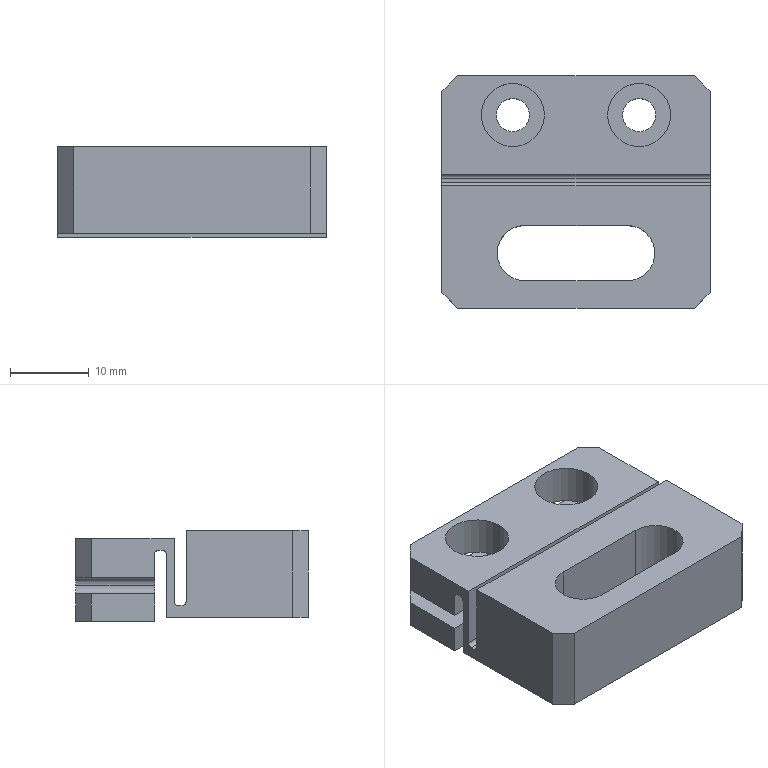Part | SolidWorks | features MoveFace 11, Cut 3, DelFace 2, Fillet 2, BaseBody 1, ICE 1 | 1 solid | 47 faces | box 34 x 29.5 x 11.5 mm | volume 7154 mm3 | plane 28 | cylinder 19 | commonest cylinder face diameters 1 x4 2 x4 4.2 x4 8 x4 7 x3
STEP:
#1=CARTESIAN_POINT('',(4.,8.75,9.));
#2=VERTEX_POINT('',#1);
#3=CARTESIAN_POINT('',(12.,8.75,9.));
#4=VERTEX_POINT('',#3);
#5=CARTESIAN_POINT('',(8.,8.75,9.));
#6=DIRECTION('',(0.,0.,1.));
#7=DIRECTION('',(1.,0.,0.));
#8=AXIS2_PLACEMENT_3D('',#5,#6,#7);
#9=CIRCLE('',#8,4.);
#10=EDGE_CURVE('',#2,#4,#9,.T.);
#11=ORIENTED_EDGE('',*,*,#10,.F.);
#12=CARTESIAN_POINT('',(4.,8.75,14.));
#13=VERTEX_POINT('',#12);
#14=CARTESIAN_POINT('',(4.,8.75,8.));
#15=DIRECTION('',(0.,0.,1.));
#16=VECTOR('',#15,1000.);
#17=LINE('',#14,#16);
#18=EDGE_CURVE('',#2,#13,#17,.T.);
#19=ORIENTED_EDGE('',*,*,#18,.T.);
#20=CARTESIAN_POINT('',(12.,8.75,14.));
#21=VERTEX_POINT('',#20);
#22=CARTESIAN_POINT('',(8.,8.75,14.));
#23=DIRECTION('',(0.,0.,1.));
#24=DIRECTION('',(1.,0.,0.));
#25=AXIS2_PLACEMENT_3D('',#22,#23,#24);
#26=CIRCLE('',#25,4.);
#27=EDGE_CURVE('',#13,#21,#26,.T.);
#28=ORIENTED_EDGE('',*,*,#27,.T.);
#29=CARTESIAN_POINT('',(12.,8.75,8.));
#30=DIRECTION('',(0.,0.,1.));
#31=VECTOR('',#30,1000.);
#32=LINE('',#29,#31);
#33=EDGE_CURVE('',#4,#21,#32,.T.);
#34=ORIENTED_EDGE('',*,*,#33,.F.);
#35=EDGE_LOOP('',(#11,#19,#28,#34));
#36=FACE_OUTER_BOUND('',#35,.T.);
#37=CARTESIAN_POINT('',(8.,8.75,8.));
#38=DIRECTION('',(0.,0.,1.));
#39=DIRECTION('',(1.,0.,0.));
#40=AXIS2_PLACEMENT_3D('',#37,#38,#39);
#41=CYLINDRICAL_SURFACE('',#40,4.);
#42=ADVANCED_FACE('',(#36),#41,.F.);
#43=CARTESIAN_POINT('',(-12.,8.75,9.));
#44=VERTEX_POINT('',#43);
#45=CARTESIAN_POINT('',(-4.,8.75,9.));
#46=VERTEX_POINT('',#45);
#47=CARTESIAN_POINT('',(-8.,8.75,9.));
#48=DIRECTION('',(0.,0.,1.));
#49=DIRECTION('',(1.,0.,0.));
#50=AXIS2_PLACEMENT_3D('',#47,#48,#49);
#51=CIRCLE('',#50,4.);
#52=EDGE_CURVE('',#44,#46,#51,.T.);
#53=ORIENTED_EDGE('',*,*,#52,.F.);
#54=CARTESIAN_POINT('',(-12.,8.75,14.));
#55=VERTEX_POINT('',#54);
#56=CARTESIAN_POINT('',(-12.,8.75,8.));
#57=DIRECTION('',(0.,0.,1.));
#58=VECTOR('',#57,1000.);
#59=LINE('',#56,#58);
#60=EDGE_CURVE('',#44,#55,#59,.T.);
#61=ORIENTED_EDGE('',*,*,#60,.T.);
#62=CARTESIAN_POINT('',(-4.,8.75,14.));
#63=VERTEX_POINT('',#62);
#64=CARTESIAN_POINT('',(-8.,8.75,14.));
#65=DIRECTION('',(0.,0.,1.));
#66=DIRECTION('',(1.,0.,0.));
#67=AXIS2_PLACEMENT_3D('',#64,#65,#66);
#68=CIRCLE('',#67,4.);
#69=EDGE_CURVE('',#55,#63,#68,.T.);
#70=ORIENTED_EDGE('',*,*,#69,.T.);
#71=CARTESIAN_POINT('',(-4.,8.75,8.));
#72=DIRECTION('',(0.,0.,1.));
#73=VECTOR('',#72,1000.);
#74=LINE('',#71,#73);
#75=EDGE_CURVE('',#46,#63,#74,.T.);
#76=ORIENTED_EDGE('',*,*,#75,.F.);
#77=EDGE_LOOP('',(#53,#61,#70,#76));
#78=FACE_OUTER_BOUND('',#77,.T.);
#79=CARTESIAN_POINT('',(-8.,8.75,8.));
#80=DIRECTION('',(0.,0.,1.));
#81=DIRECTION('',(1.,0.,0.));
#82=AXIS2_PLACEMENT_3D('',#79,#80,#81);
#83=CYLINDRICAL_SURFACE('',#82,4.);
#84=ADVANCED_FACE('',(#78),#83,.F.);
#85=CARTESIAN_POINT('',(-5.9,8.75,3.5));
#86=VERTEX_POINT('',#85);
#87=CARTESIAN_POINT('',(-10.1,8.75,3.5));
#88=VERTEX_POINT('',#87);
#89=CARTESIAN_POINT('',(-8.,8.75,3.5));
#90=DIRECTION('',(0.,0.,-1.));
#91=DIRECTION('',(-1.,0.,0.));
#92=AXIS2_PLACEMENT_3D('',#89,#90,#91);
#93=CIRCLE('',#92,2.1);
#94=EDGE_CURVE('',#86,#88,#93,.T.);
#95=ORIENTED_EDGE('',*,*,#94,.T.);
#96=CARTESIAN_POINT('',(-10.1,8.75,7.));
#97=VERTEX_POINT('',#96);
#98=CARTESIAN_POINT('',(-10.1,8.75,-6.));
#99=DIRECTION('',(0.,0.,1.));
#100=VECTOR('',#99,1000.);
#101=LINE('',#98,#100);
#102=EDGE_CURVE('',#88,#97,#101,.T.);
#103=ORIENTED_EDGE('',*,*,#102,.T.);
#104=CARTESIAN_POINT('',(-5.9,8.75,7.));
#105=VERTEX_POINT('',#104);
#106=CARTESIAN_POINT('',(-8.,8.75,7.));
#107=DIRECTION('',(0.,0.,-1.));
#108=DIRECTION('',(-1.,0.,0.));
#109=AXIS2_PLACEMENT_3D('',#106,#107,#108);
#110=CIRCLE('',#109,2.1);
#111=EDGE_CURVE('',#105,#97,#110,.T.);
#112=ORIENTED_EDGE('',*,*,#111,.F.);
#113=CARTESIAN_POINT('',(-5.9,8.75,-6.));
#114=DIRECTION('',(0.,0.,1.));
#115=VECTOR('',#114,1000.);
#116=LINE('',#113,#115);
#117=EDGE_CURVE('',#86,#105,#116,.T.);
#118=ORIENTED_EDGE('',*,*,#117,.F.);
#119=EDGE_LOOP('',(#95,#103,#112,#118));
#120=FACE_OUTER_BOUND('',#119,.T.);
#121=CARTESIAN_POINT('',(-8.,8.75,-6.));
#122=DIRECTION('',(0.,0.,1.));
#123=DIRECTION('',(1.,0.,0.));
#124=AXIS2_PLACEMENT_3D('',#121,#122,#123);
#125=CYLINDRICAL_SURFACE('',#124,2.1);
#126=ADVANCED_FACE('',(#120),#125,.F.);
#127=CARTESIAN_POINT('',(10.1,8.75,3.5));
#128=VERTEX_POINT('',#127);
#129=CARTESIAN_POINT('',(5.9,8.75,3.5));
#130=VERTEX_POINT('',#129);
#131=CARTESIAN_POINT('',(8.,8.75,3.5));
#132=DIRECTION('',(0.,0.,-1.));
#133=DIRECTION('',(-1.,0.,0.));
#134=AXIS2_PLACEMENT_3D('',#131,#132,#133);
#135=CIRCLE('',#134,2.1);
#136=EDGE_CURVE('',#128,#130,#135,.T.);
#137=ORIENTED_EDGE('',*,*,#136,.T.);
#138=CARTESIAN_POINT('',(5.9,8.75,7.));
#139=VERTEX_POINT('',#138);
#140=CARTESIAN_POINT('',(5.9,8.75,-6.));
#141=DIRECTION('',(0.,0.,1.));
#142=VECTOR('',#141,1000.);
#143=LINE('',#140,#142);
#144=EDGE_CURVE('',#130,#139,#143,.T.);
#145=ORIENTED_EDGE('',*,*,#144,.T.);
#146=CARTESIAN_POINT('',(10.1,8.75,7.));
#147=VERTEX_POINT('',#146);
#148=CARTESIAN_POINT('',(8.,8.75,7.));
#149=DIRECTION('',(0.,0.,-1.));
#150=DIRECTION('',(-1.,0.,0.));
#151=AXIS2_PLACEMENT_3D('',#148,#149,#150);
#152=CIRCLE('',#151,2.1);
#153=EDGE_CURVE('',#147,#139,#152,.T.);
#154=ORIENTED_EDGE('',*,*,#153,.F.);
#155=CARTESIAN_POINT('',(10.1,8.75,-6.));
#156=DIRECTION('',(0.,0.,1.));
#157=VECTOR('',#156,1000.);
#158=LINE('',#155,#157);
#159=EDGE_CURVE('',#128,#147,#158,.T.);
#160=ORIENTED_EDGE('',*,*,#159,.F.);
#161=EDGE_LOOP('',(#137,#145,#154,#160));
#162=FACE_OUTER_BOUND('',#161,.T.);
#163=CARTESIAN_POINT('',(8.,8.75,-6.));
#164=DIRECTION('',(0.,0.,1.));
#165=DIRECTION('',(1.,0.,0.));
#166=AXIS2_PLACEMENT_3D('',#163,#164,#165);
#167=CYLINDRICAL_SURFACE('',#166,2.1);
#168=ADVANCED_FACE('',(#162),#167,.F.);
#169=CARTESIAN_POINT('',(-6.5,-5.25,15.));
#170=VERTEX_POINT('',#169);
#171=CARTESIAN_POINT('',(-10.,-8.75,15.));
#172=VERTEX_POINT('',#171);
#173=CARTESIAN_POINT('',(-6.5,-8.75,15.));
#174=DIRECTION('',(0.,0.,1.));
#175=DIRECTION('',(-1.,0.,0.));
#176=AXIS2_PLACEMENT_3D('',#173,#174,#175);
#177=CIRCLE('',#176,3.5);
#178=EDGE_CURVE('',#170,#172,#177,.T.);
#179=ORIENTED_EDGE('',*,*,#178,.T.);
#180=CARTESIAN_POINT('',(-10.,-8.75,4.));
#181=VERTEX_POINT('',#180);
#182=CARTESIAN_POINT('',(-10.,-8.75,18.));
#183=DIRECTION('',(0.,0.,-1.));
#184=VECTOR('',#183,1000.);
#185=LINE('',#182,#184);
#186=EDGE_CURVE('',#172,#181,#185,.T.);
#187=ORIENTED_EDGE('',*,*,#186,.T.);
#188=CARTESIAN_POINT('',(-6.5,-5.25,4.));
#189=VERTEX_POINT('',#188);
#190=CARTESIAN_POINT('',(-6.5,-8.75,4.));
#191=DIRECTION('',(0.,0.,-1.));
#192=DIRECTION('',(1.,0.,0.));
#193=AXIS2_PLACEMENT_3D('',#190,#191,#192);
#194=CIRCLE('',#193,3.5);
#195=EDGE_CURVE('',#181,#189,#194,.T.);
#196=ORIENTED_EDGE('',*,*,#195,.T.);
#197=CARTESIAN_POINT('',(-6.5,-5.25,18.));
#198=DIRECTION('',(0.,0.,-1.));
#199=VECTOR('',#198,1000.);
#200=LINE('',#197,#199);
#201=EDGE_CURVE('',#170,#189,#200,.T.);
#202=ORIENTED_EDGE('',*,*,#201,.F.);
#203=EDGE_LOOP('',(#179,#187,#196,#202));
#204=FACE_OUTER_BOUND('',#203,.T.);
#205=CARTESIAN_POINT('',(-6.5,-8.75,18.));
#206=DIRECTION('',(0.,0.,-1.));
#207=DIRECTION('',(-1.,0.,0.));
#208=AXIS2_PLACEMENT_3D('',#205,#206,#207);
#209=CYLINDRICAL_SURFACE('',#208,3.5);
#210=ADVANCED_FACE('',(#204),#209,.F.);
#211=CARTESIAN_POINT('',(8.,8.75,14.));
#212=DIRECTION('',(0.,0.,1.));
#213=DIRECTION('',(1.,0.,0.));
#214=AXIS2_PLACEMENT_3D('',#211,#212,#213);
#215=CIRCLE('',#214,4.);
#216=EDGE_CURVE('',#21,#13,#215,.T.);
#217=ORIENTED_EDGE('',*,*,#216,.F.);
#218=ORIENTED_EDGE('',*,*,#27,.F.);
#219=EDGE_LOOP('',(#217,#218));
#220=FACE_BOUND('',#219,.T.);
#221=CARTESIAN_POINT('',(-8.,8.75,14.));
#222=DIRECTION('',(0.,0.,1.));
#223=DIRECTION('',(1.,0.,0.));
#224=AXIS2_PLACEMENT_3D('',#221,#222,#223);
#225=CIRCLE('',#224,4.);
#226=EDGE_CURVE('',#63,#55,#225,.T.);
#227=ORIENTED_EDGE('',*,*,#226,.F.);
#228=ORIENTED_EDGE('',*,*,#69,.F.);
#229=EDGE_LOOP('',(#227,#228));
#230=FACE_BOUND('',#229,.T.);
#231=CARTESIAN_POINT('',(15.,13.75,14.));
#232=VERTEX_POINT('',#231);
#233=CARTESIAN_POINT('',(17.,11.75,14.));
#234=VERTEX_POINT('',#233);
#235=CARTESIAN_POINT('',(15.,13.75,14.));
#236=DIRECTION('',(0.7071,-0.7071,0.));
#237=VECTOR('',#236,1000.);
#238=LINE('',#235,#237);
#239=EDGE_CURVE('',#232,#234,#238,.T.);
#240=ORIENTED_EDGE('',*,*,#239,.F.);
#241=CARTESIAN_POINT('',(-15.,13.75,14.));
#242=VERTEX_POINT('',#241);
#243=CARTESIAN_POINT('',(-50.,13.75,14.));
#244=DIRECTION('',(1.,0.,0.));
#245=VECTOR('',#244,1000.);
#246=LINE('',#243,#245);
#247=EDGE_CURVE('',#242,#232,#246,.T.);
#248=ORIENTED_EDGE('',*,*,#247,.F.);
#249=CARTESIAN_POINT('',(-17.,11.75,14.));
#250=VERTEX_POINT('',#249);
#251=CARTESIAN_POINT('',(-17.,11.75,14.));
#252=DIRECTION('',(0.7071,0.7071,0.));
#253=VECTOR('',#252,1000.);
#254=LINE('',#251,#253);
#255=EDGE_CURVE('',#250,#242,#254,.T.);
#256=ORIENTED_EDGE('',*,*,#255,.F.);
#257=CARTESIAN_POINT('',(-17.,1.25,14.));
#258=VERTEX_POINT('',#257);
#259=CARTESIAN_POINT('',(-17.,18.75,14.));
#260=DIRECTION('',(0.,1.,0.));
#261=VECTOR('',#260,1000.);
#262=LINE('',#259,#261);
#263=EDGE_CURVE('',#258,#250,#262,.T.);
#264=ORIENTED_EDGE('',*,*,#263,.F.);
#265=CARTESIAN_POINT('',(17.,1.25,14.));
#266=VERTEX_POINT('',#265);
#267=CARTESIAN_POINT('',(-50.,1.25,14.));
#268=DIRECTION('',(-1.,0.,0.));
#269=VECTOR('',#268,1000.);
#270=LINE('',#267,#269);
#271=EDGE_CURVE('',#266,#258,#270,.T.);
#272=ORIENTED_EDGE('',*,*,#271,.F.);
#273=CARTESIAN_POINT('',(17.,18.75,14.));
#274=DIRECTION('',(0.,-1.,0.));
#275=VECTOR('',#274,1000.);
#276=LINE('',#273,#275);
#277=EDGE_CURVE('',#234,#266,#276,.T.);
#278=ORIENTED_EDGE('',*,*,#277,.F.);
#279=EDGE_LOOP('',(#240,#248,#256,#264,#272,#278));
#280=FACE_OUTER_BOUND('',#279,.T.);
#281=CARTESIAN_POINT('',(-50.,18.75,14.));
#282=DIRECTION('',(0.,0.,-1.));
#283=DIRECTION('',(0.,1.,0.));
#284=AXIS2_PLACEMENT_3D('',#281,#282,#283);
#285=PLANE('',#284);
#286=ADVANCED_FACE('',(#220,#230,#280),#285,.F.);
#287=CARTESIAN_POINT('',(17.,-13.75,4.));
#288=VERTEX_POINT('',#287);
#289=CARTESIAN_POINT('',(17.,-13.75,15.));
#290=VERTEX_POINT('',#289);
#291=CARTESIAN_POINT('',(17.,-13.75,18.));
#292=DIRECTION('',(0.,0.,1.));
#293=VECTOR('',#292,1000.);
#294=LINE('',#291,#293);
#295=EDGE_CURVE('',#288,#290,#294,.T.);
#296=ORIENTED_EDGE('',*,*,#295,.F.);
#297=CARTESIAN_POINT('',(17.,2.25,4.));
#298=VERTEX_POINT('',#297);
#299=CARTESIAN_POINT('',(17.,2.25,4.));
#300=DIRECTION('',(0.,-1.,0.));
#301=VECTOR('',#300,1000.);
#302=LINE('',#299,#301);
#303=EDGE_CURVE('',#298,#288,#302,.T.);
#304=ORIENTED_EDGE('',*,*,#303,.F.);
#305=CARTESIAN_POINT('',(17.,2.25,12.));
#306=VERTEX_POINT('',#305);
#307=CARTESIAN_POINT('',(17.,2.25,18.));
#308=DIRECTION('',(0.,0.,-1.));
#309=VECTOR('',#308,1000.);
#310=LINE('',#307,#309);
#311=EDGE_CURVE('',#306,#298,#310,.T.);
#312=ORIENTED_EDGE('',*,*,#311,.F.);
#313=CARTESIAN_POINT('',(17.,2.75,12.5));
#314=VERTEX_POINT('',#313);
#315=CARTESIAN_POINT('',(17.,2.75,12.));
#316=DIRECTION('',(-1.,0.,0.));
#317=DIRECTION('',(0.,0.,1.));
#318=AXIS2_PLACEMENT_3D('',#315,#316,#317);
#319=CIRCLE('',#318,0.5);
#320=EDGE_CURVE('',#306,#314,#319,.T.);
#321=ORIENTED_EDGE('',*,*,#320,.T.);
#322=CARTESIAN_POINT('',(17.,3.25,12.5));
#323=VERTEX_POINT('',#322);
#324=CARTESIAN_POINT('',(17.,3.75,12.5));
#325=DIRECTION('',(0.,1.,0.));
#326=VECTOR('',#325,1000.);
#327=LINE('',#324,#326);
#328=EDGE_CURVE('',#314,#323,#327,.T.);
#329=ORIENTED_EDGE('',*,*,#328,.T.);
#330=CARTESIAN_POINT('',(17.,3.75,12.));
#331=VERTEX_POINT('',#330);
#332=CARTESIAN_POINT('',(17.,3.25,12.));
#333=DIRECTION('',(-1.,0.,0.));
#334=DIRECTION('',(0.,0.,1.));
#335=AXIS2_PLACEMENT_3D('',#332,#333,#334);
#336=CIRCLE('',#335,0.5);
#337=EDGE_CURVE('',#323,#331,#336,.T.);
#338=ORIENTED_EDGE('',*,*,#337,.T.);
#339=CARTESIAN_POINT('',(17.,3.75,9.));
#340=VERTEX_POINT('',#339);
#341=CARTESIAN_POINT('',(17.,3.75,18.));
#342=DIRECTION('',(0.,0.,1.));
#343=VECTOR('',#342,1000.);
#344=LINE('',#341,#343);
#345=EDGE_CURVE('',#340,#331,#344,.T.);
#346=ORIENTED_EDGE('',*,*,#345,.F.);
#347=CARTESIAN_POINT('',(17.,11.75,9.));
#348=VERTEX_POINT('',#347);
#349=CARTESIAN_POINT('',(17.,-18.75,9.));
#350=DIRECTION('',(0.,-1.,0.));
#351=VECTOR('',#350,1000.);
#352=LINE('',#349,#351);
#353=EDGE_CURVE('',#348,#340,#352,.T.);
#354=ORIENTED_EDGE('',*,*,#353,.F.);
#355=CARTESIAN_POINT('',(17.,11.75,18.));
#356=DIRECTION('',(0.,0.,-1.));
#357=VECTOR('',#356,1000.);
#358=LINE('',#355,#357);
#359=EDGE_CURVE('',#234,#348,#358,.T.);
#360=ORIENTED_EDGE('',*,*,#359,.F.);
#361=ORIENTED_EDGE('',*,*,#277,.T.);
#362=CARTESIAN_POINT('',(17.,1.25,6.));
#363=VERTEX_POINT('',#362);
#364=CARTESIAN_POINT('',(17.,1.25,18.));
#365=DIRECTION('',(0.,0.,1.));
#366=VECTOR('',#365,1000.);
#367=LINE('',#364,#366);
#368=EDGE_CURVE('',#363,#266,#367,.T.);
#369=ORIENTED_EDGE('',*,*,#368,.F.);
#370=CARTESIAN_POINT('',(17.,0.75,5.5));
#371=VERTEX_POINT('',#370);
#372=CARTESIAN_POINT('',(17.,0.75,6.));
#373=DIRECTION('',(-1.,0.,0.));
#374=DIRECTION('',(0.,0.,1.));
#375=AXIS2_PLACEMENT_3D('',#372,#373,#374);
#376=CIRCLE('',#375,0.5);
#377=EDGE_CURVE('',#363,#371,#376,.T.);
#378=ORIENTED_EDGE('',*,*,#377,.T.);
#379=CARTESIAN_POINT('',(17.,0.25,5.5));
#380=VERTEX_POINT('',#379);
#381=CARTESIAN_POINT('',(17.,0.75,5.5));
#382=DIRECTION('',(0.,-1.,0.));
#383=VECTOR('',#382,1000.);
#384=LINE('',#381,#383);
#385=EDGE_CURVE('',#371,#380,#384,.T.);
#386=ORIENTED_EDGE('',*,*,#385,.T.);
#387=CARTESIAN_POINT('',(17.,-0.25,6.));
#388=VERTEX_POINT('',#387);
#389=CARTESIAN_POINT('',(17.,0.25,6.));
#390=DIRECTION('',(-1.,0.,0.));
#391=DIRECTION('',(0.,0.,1.));
#392=AXIS2_PLACEMENT_3D('',#389,#390,#391);
#393=CIRCLE('',#392,0.5);
#394=EDGE_CURVE('',#380,#388,#393,.T.);
#395=ORIENTED_EDGE('',*,*,#394,.T.);
#396=CARTESIAN_POINT('',(17.,-0.25,15.));
#397=VERTEX_POINT('',#396);
#398=CARTESIAN_POINT('',(17.,-0.25,18.));
#399=DIRECTION('',(0.,0.,-1.));
#400=VECTOR('',#399,1000.);
#401=LINE('',#398,#400);
#402=EDGE_CURVE('',#397,#388,#401,.T.);
#403=ORIENTED_EDGE('',*,*,#402,.F.);
#404=CARTESIAN_POINT('',(17.,-18.75,15.));
#405=DIRECTION('',(0.,1.,0.));
#406=VECTOR('',#405,1000.);
#407=LINE('',#404,#406);
#408=EDGE_CURVE('',#290,#397,#407,.T.);
#409=ORIENTED_EDGE('',*,*,#408,.F.);
#410=EDGE_LOOP('',(#296,#304,#312,#321,#329,#338,#346,#354,#360,#361,#369,#378,#386,#395,#403,#409));
#411=FACE_OUTER_BOUND('',#410,.T.);
#412=CARTESIAN_POINT('',(17.,-18.75,18.));
#413=DIRECTION('',(-1.,0.,0.));
#414=DIRECTION('',(0.,0.,1.));
#415=AXIS2_PLACEMENT_3D('',#412,#413,#414);
#416=PLANE('',#415);
#417=ADVANCED_FACE('',(#411),#416,.F.);
#418=CARTESIAN_POINT('',(15.,13.75,9.));
#419=VERTEX_POINT('',#418);
#420=CARTESIAN_POINT('',(15.,13.75,9.));
#421=DIRECTION('',(0.7071,-0.7071,0.));
#422=VECTOR('',#421,1000.);
#423=LINE('',#420,#422);
#424=EDGE_CURVE('',#419,#348,#423,.T.);
#425=ORIENTED_EDGE('',*,*,#424,.F.);
#426=CARTESIAN_POINT('',(15.,13.75,18.));
#427=DIRECTION('',(0.,0.,-1.));
#428=VECTOR('',#427,1000.);
#429=LINE('',#426,#428);
#430=EDGE_CURVE('',#232,#419,#429,.T.);
#431=ORIENTED_EDGE('',*,*,#430,.F.);
#432=ORIENTED_EDGE('',*,*,#239,.T.);
#433=ORIENTED_EDGE('',*,*,#359,.T.);
#434=EDGE_LOOP('',(#425,#431,#432,#433));
#435=FACE_OUTER_BOUND('',#434,.T.);
#436=CARTESIAN_POINT('',(15.,13.75,18.));
#437=DIRECTION('',(-0.7071,-0.7071,0.));
#438=DIRECTION('',(0.7071,-0.7071,0.));
#439=AXIS2_PLACEMENT_3D('',#436,#437,#438);
#440=PLANE('',#439);
#441=ADVANCED_FACE('',(#435),#440,.F.);
#442=CARTESIAN_POINT('',(2.5,13.75,9.));
#443=VERTEX_POINT('',#442);
#444=CARTESIAN_POINT('',(1.5,13.75,8.));
#445=VERTEX_POINT('',#444);
#446=CARTESIAN_POINT('',(2.5,13.75,8.));
#447=DIRECTION('',(0.,-1.,0.));
#448=DIRECTION('',(0.,0.,-1.));
#449=AXIS2_PLACEMENT_3D('',#446,#447,#448);
#450=CIRCLE('',#449,1.);
#451=EDGE_CURVE('',#443,#445,#450,.T.);
#452=ORIENTED_EDGE('',*,*,#451,.T.);
#453=CARTESIAN_POINT('',(2.5,13.75,7.));
#454=VERTEX_POINT('',#453);
#455=CARTESIAN_POINT('',(2.5,13.75,8.));
#456=DIRECTION('',(0.,-1.,0.));
#457=DIRECTION('',(0.,0.,-1.));
#458=AXIS2_PLACEMENT_3D('',#455,#456,#457);
#459=CIRCLE('',#458,1.);
#460=EDGE_CURVE('',#445,#454,#459,.T.);
#461=ORIENTED_EDGE('',*,*,#460,.T.);
#462=CARTESIAN_POINT('',(15.,13.75,7.));
#463=VERTEX_POINT('',#462);
#464=CARTESIAN_POINT('',(-20.,13.75,7.));
#465=DIRECTION('',(-1.,0.,0.));
#466=VECTOR('',#465,1000.);
#467=LINE('',#464,#466);
#468=EDGE_CURVE('',#463,#454,#467,.T.);
#469=ORIENTED_EDGE('',*,*,#468,.F.);
#470=CARTESIAN_POINT('',(15.,13.75,3.5));
#471=VERTEX_POINT('',#470);
#472=CARTESIAN_POINT('',(15.,13.75,18.));
#473=DIRECTION('',(0.,0.,1.));
#474=VECTOR('',#473,1000.);
#475=LINE('',#472,#474);
#476=EDGE_CURVE('',#471,#463,#475,.T.);
#477=ORIENTED_EDGE('',*,*,#476,.F.);
#478=CARTESIAN_POINT('',(-15.,13.75,3.5));
#479=VERTEX_POINT('',#478);
#480=CARTESIAN_POINT('',(-20.,13.75,3.5));
#481=DIRECTION('',(1.,0.,0.));
#482=VECTOR('',#481,1000.);
#483=LINE('',#480,#482);
#484=EDGE_CURVE('',#479,#471,#483,.T.);
#485=ORIENTED_EDGE('',*,*,#484,.F.);
#486=CARTESIAN_POINT('',(-15.,13.75,7.));
#487=VERTEX_POINT('',#486);
#488=CARTESIAN_POINT('',(-15.,13.75,18.));
#489=DIRECTION('',(0.,0.,-1.));
#490=VECTOR('',#489,1000.);
#491=LINE('',#488,#490);
#492=EDGE_CURVE('',#487,#479,#491,.T.);
#493=ORIENTED_EDGE('',*,*,#492,.F.);
#494=CARTESIAN_POINT('',(-2.5,13.75,7.));
#495=VERTEX_POINT('',#494);
#496=CARTESIAN_POINT('',(-20.,13.75,7.));
#497=DIRECTION('',(-1.,0.,0.));
#498=VECTOR('',#497,1000.);
#499=LINE('',#496,#498);
#500=EDGE_CURVE('',#495,#487,#499,.T.);
#501=ORIENTED_EDGE('',*,*,#500,.F.);
#502=CARTESIAN_POINT('',(-1.5,13.75,8.));
#503=VERTEX_POINT('',#502);
#504=CARTESIAN_POINT('',(-2.5,13.75,8.));
#505=DIRECTION('',(0.,-1.,0.));
#506=DIRECTION('',(0.,0.,-1.));
#507=AXIS2_PLACEMENT_3D('',#504,#505,#506);
#508=CIRCLE('',#507,1.);
#509=EDGE_CURVE('',#495,#503,#508,.T.);
#510=ORIENTED_EDGE('',*,*,#509,.T.);
#511=CARTESIAN_POINT('',(-2.5,13.75,9.));
#512=VERTEX_POINT('',#511);
#513=CARTESIAN_POINT('',(-2.5,13.75,8.));
#514=DIRECTION('',(0.,-1.,0.));
#515=DIRECTION('',(0.,0.,-1.));
#516=AXIS2_PLACEMENT_3D('',#513,#514,#515);
#517=CIRCLE('',#516,1.);
#518=EDGE_CURVE('',#503,#512,#517,.T.);
#519=ORIENTED_EDGE('',*,*,#518,.T.);
#520=CARTESIAN_POINT('',(-15.,13.75,9.));
#521=VERTEX_POINT('',#520);
#522=CARTESIAN_POINT('',(-20.,13.75,9.));
#523=DIRECTION('',(1.,0.,0.));
#524=VECTOR('',#523,1000.);
#525=LINE('',#522,#524);
#526=EDGE_CURVE('',#521,#512,#525,.T.);
#527=ORIENTED_EDGE('',*,*,#526,.F.);
#528=CARTESIAN_POINT('',(-15.,13.75,18.));
#529=DIRECTION('',(0.,0.,-1.));
#530=VECTOR('',#529,1000.);
#531=LINE('',#528,#530);
#532=EDGE_CURVE('',#242,#521,#531,.T.);
#533=ORIENTED_EDGE('',*,*,#532,.F.);
#534=ORIENTED_EDGE('',*,*,#247,.T.);
#535=ORIENTED_EDGE('',*,*,#430,.T.);
#536=CARTESIAN_POINT('',(-20.,13.75,9.));
#537=DIRECTION('',(1.,0.,0.));
#538=VECTOR('',#537,1000.);
#539=LINE('',#536,#538);
#540=EDGE_CURVE('',#443,#419,#539,.T.);
#541=ORIENTED_EDGE('',*,*,#540,.F.);
#542=EDGE_LOOP('',(#452,#461,#469,#477,#485,#493,#501,#510,#519,#527,#533,#534,#535,#541));
#543=FACE_OUTER_BOUND('',#542,.T.);
#544=CARTESIAN_POINT('',(-20.,13.75,18.));
#545=DIRECTION('',(0.,-1.,0.));
#546=DIRECTION('',(0.,0.,-1.));
#547=AXIS2_PLACEMENT_3D('',#544,#545,#546);
#548=PLANE('',#547);
#549=ADVANCED_FACE('',(#543),#548,.F.);
#550=CARTESIAN_POINT('',(-17.,11.75,9.));
#551=VERTEX_POINT('',#550);
#552=CARTESIAN_POINT('',(-17.,11.75,9.));
#553=DIRECTION('',(0.7071,0.7071,0.));
#554=VECTOR('',#553,1000.);
#555=LINE('',#552,#554);
#556=EDGE_CURVE('',#551,#521,#555,.T.);
#557=ORIENTED_EDGE('',*,*,#556,.F.);
#558=CARTESIAN_POINT('',(-17.,11.75,18.));
#559=DIRECTION('',(0.,0.,-1.));
#560=VECTOR('',#559,1000.);
#561=LINE('',#558,#560);
#562=EDGE_CURVE('',#250,#551,#561,.T.);
#563=ORIENTED_EDGE('',*,*,#562,.F.);
#564=ORIENTED_EDGE('',*,*,#255,.T.);
#565=ORIENTED_EDGE('',*,*,#532,.T.);
#566=EDGE_LOOP('',(#557,#563,#564,#565));
#567=FACE_OUTER_BOUND('',#566,.T.);
#568=CARTESIAN_POINT('',(-17.,11.75,18.));
#569=DIRECTION('',(0.7071,-0.7071,0.));
#570=DIRECTION('',(0.7071,0.7071,0.));
#571=AXIS2_PLACEMENT_3D('',#568,#569,#570);
#572=PLANE('',#571);
#573=ADVANCED_FACE('',(#567),#572,.F.);
#574=CARTESIAN_POINT('',(-17.,2.25,4.));
#575=VERTEX_POINT('',#574);
#576=CARTESIAN_POINT('',(-17.,2.25,12.));
#577=VERTEX_POINT('',#576);
#578=CARTESIAN_POINT('',(-17.,2.25,18.));
#579=DIRECTION('',(0.,0.,1.));
#580=VECTOR('',#579,1000.);
#581=LINE('',#578,#580);
#582=EDGE_CURVE('',#575,#577,#581,.T.);
#583=ORIENTED_EDGE('',*,*,#582,.F.);
#584=CARTESIAN_POINT('',(-17.,-13.75,4.));
#585=VERTEX_POINT('',#584);
#586=CARTESIAN_POINT('',(-17.,-18.75,4.));
#587=DIRECTION('',(0.,-1.,0.));
#588=VECTOR('',#587,1000.);
#589=LINE('',#586,#588);
#590=EDGE_CURVE('',#575,#585,#589,.T.);
#591=ORIENTED_EDGE('',*,*,#590,.T.);
#592=CARTESIAN_POINT('',(-17.,-13.75,15.));
#593=VERTEX_POINT('',#592);
#594=CARTESIAN_POINT('',(-17.,-13.75,18.));
#595=DIRECTION('',(0.,0.,-1.));
#596=VECTOR('',#595,1000.);
#597=LINE('',#594,#596);
#598=EDGE_CURVE('',#593,#585,#597,.T.);
#599=ORIENTED_EDGE('',*,*,#598,.F.);
#600=CARTESIAN_POINT('',(-17.,-0.25,15.));
#601=VERTEX_POINT('',#600);
#602=CARTESIAN_POINT('',(-17.,-18.75,15.));
#603=DIRECTION('',(0.,-1.,0.));
#604=VECTOR('',#603,1000.);
#605=LINE('',#602,#604);
#606=EDGE_CURVE('',#601,#593,#605,.T.);
#607=ORIENTED_EDGE('',*,*,#606,.F.);
#608=CARTESIAN_POINT('',(-17.,-0.25,6.));
#609=VERTEX_POINT('',#608);
#610=CARTESIAN_POINT('',(-17.,-0.25,18.));
#611=DIRECTION('',(0.,0.,1.));
#612=VECTOR('',#611,1000.);
#613=LINE('',#610,#612);
#614=EDGE_CURVE('',#609,#601,#613,.T.);
#615=ORIENTED_EDGE('',*,*,#614,.F.);
#616=CARTESIAN_POINT('',(-17.,0.25,5.5));
#617=VERTEX_POINT('',#616);
#618=CARTESIAN_POINT('',(-17.,0.25,6.));
#619=DIRECTION('',(1.,0.,0.));
#620=DIRECTION('',(0.,0.,-1.));
#621=AXIS2_PLACEMENT_3D('',#618,#619,#620);
#622=CIRCLE('',#621,0.5);
#623=EDGE_CURVE('',#609,#617,#622,.T.);
#624=ORIENTED_EDGE('',*,*,#623,.T.);
#625=CARTESIAN_POINT('',(-17.,0.75,5.5));
#626=VERTEX_POINT('',#625);
#627=CARTESIAN_POINT('',(-17.,0.75,5.5));
#628=DIRECTION('',(0.,1.,0.));
#629=VECTOR('',#628,1000.);
#630=LINE('',#627,#629);
#631=EDGE_CURVE('',#617,#626,#630,.T.);
#632=ORIENTED_EDGE('',*,*,#631,.T.);
#633=CARTESIAN_POINT('',(-17.,1.25,6.));
#634=VERTEX_POINT('',#633);
#635=CARTESIAN_POINT('',(-17.,0.75,6.));
#636=DIRECTION('',(1.,0.,0.));
#637=DIRECTION('',(0.,0.,-1.));
#638=AXIS2_PLACEMENT_3D('',#635,#636,#637);
#639=CIRCLE('',#638,0.5);
#640=EDGE_CURVE('',#626,#634,#639,.T.);
#641=ORIENTED_EDGE('',*,*,#640,.T.);
#642=CARTESIAN_POINT('',(-17.,1.25,18.));
#643=DIRECTION('',(0.,0.,-1.));
#644=VECTOR('',#643,1000.);
#645=LINE('',#642,#644);
#646=EDGE_CURVE('',#258,#634,#645,.T.);
#647=ORIENTED_EDGE('',*,*,#646,.F.);
#648=ORIENTED_EDGE('',*,*,#263,.T.);
#649=ORIENTED_EDGE('',*,*,#562,.T.);
#650=CARTESIAN_POINT('',(-17.,3.75,9.));
#651=VERTEX_POINT('',#650);
#652=CARTESIAN_POINT('',(-17.,-18.75,9.));
#653=DIRECTION('',(0.,1.,0.));
#654=VECTOR('',#653,1000.);
#655=LINE('',#652,#654);
#656=EDGE_CURVE('',#651,#551,#655,.T.);
#657=ORIENTED_EDGE('',*,*,#656,.F.);
#658=CARTESIAN_POINT('',(-17.,3.75,12.));
#659=VERTEX_POINT('',#658);
#660=CARTESIAN_POINT('',(-17.,3.75,18.));
#661=DIRECTION('',(0.,0.,-1.));
#662=VECTOR('',#661,1000.);
#663=LINE('',#660,#662);
#664=EDGE_CURVE('',#659,#651,#663,.T.);
#665=ORIENTED_EDGE('',*,*,#664,.F.);
#666=CARTESIAN_POINT('',(-17.,3.25,12.5));
#667=VERTEX_POINT('',#666);
#668=CARTESIAN_POINT('',(-17.,3.25,12.));
#669=DIRECTION('',(1.,0.,0.));
#670=DIRECTION('',(0.,0.,-1.));
#671=AXIS2_PLACEMENT_3D('',#668,#669,#670);
#672=CIRCLE('',#671,0.5);
#673=EDGE_CURVE('',#659,#667,#672,.T.);
#674=ORIENTED_EDGE('',*,*,#673,.T.);
#675=CARTESIAN_POINT('',(-17.,2.75,12.5));
#676=VERTEX_POINT('',#675);
#677=CARTESIAN_POINT('',(-17.,3.75,12.5));
#678=DIRECTION('',(0.,-1.,0.));
#679=VECTOR('',#678,1000.);
#680=LINE('',#677,#679);
#681=EDGE_CURVE('',#667,#676,#680,.T.);
#682=ORIENTED_EDGE('',*,*,#681,.T.);
#683=CARTESIAN_POINT('',(-17.,2.75,12.));
#684=DIRECTION('',(1.,0.,0.));
#685=DIRECTION('',(0.,0.,-1.));
#686=AXIS2_PLACEMENT_3D('',#683,#684,#685);
#687=CIRCLE('',#686,0.5);
#688=EDGE_CURVE('',#676,#577,#687,.T.);
#689=ORIENTED_EDGE('',*,*,#688,.T.);
#690=EDGE_LOOP('',(#583,#591,#599,#607,#615,#624,#632,#641,#647,#648,#649,#657,#665,#674,#682,#689));
#691=FACE_OUTER_BOUND('',#690,.T.);
#692=CARTESIAN_POINT('',(-17.,-18.75,18.));
#693=DIRECTION('',(1.,0.,0.));
#694=DIRECTION('',(0.,0.,-1.));
#695=AXIS2_PLACEMENT_3D('',#692,#693,#694);
#696=PLANE('',#695);
#697=ADVANCED_FACE('',(#691),#696,.F.);
#698=ORIENTED_EDGE('',*,*,#646,.T.);
#699=CARTESIAN_POINT('',(-50.,1.25,6.));
#700=DIRECTION('',(1.,0.,0.));
#701=VECTOR('',#700,1000.);
#702=LINE('',#699,#701);
#703=EDGE_CURVE('',#634,#363,#702,.T.);
#704=ORIENTED_EDGE('',*,*,#703,.T.);
#705=ORIENTED_EDGE('',*,*,#368,.T.);
#706=ORIENTED_EDGE('',*,*,#271,.T.);
#707=EDGE_LOOP('',(#698,#704,#705,#706));
#708=FACE_OUTER_BOUND('',#707,.T.);
#709=CARTESIAN_POINT('',(-50.,1.25,17.));
#710=DIRECTION('',(0.,1.,0.));
#711=DIRECTION('',(0.,0.,1.));
#712=AXIS2_PLACEMENT_3D('',#709,#710,#711);
#713=PLANE('',#712);
#714=ADVANCED_FACE('',(#708),#713,.F.);
#715=CARTESIAN_POINT('',(8.,8.75,9.));
#716=DIRECTION('',(0.,0.,1.));
#717=DIRECTION('',(1.,0.,0.));
#718=AXIS2_PLACEMENT_3D('',#715,#716,#717);
#719=CIRCLE('',#718,4.);
#720=EDGE_CURVE('',#4,#2,#719,.T.);
#721=ORIENTED_EDGE('',*,*,#720,.T.);
#722=ORIENTED_EDGE('',*,*,#10,.T.);
#723=EDGE_LOOP('',(#721,#722));
#724=FACE_BOUND('',#723,.T.);
#725=CARTESIAN_POINT('',(2.5,3.75,9.));
#726=VERTEX_POINT('',#725);
#727=CARTESIAN_POINT('',(20.707,3.75,9.));
#728=DIRECTION('',(1.,0.,0.));
#729=VECTOR('',#728,1000.);
#730=LINE('',#727,#729);
#731=EDGE_CURVE('',#726,#340,#730,.T.);
#732=ORIENTED_EDGE('',*,*,#731,.F.);
#733=CARTESIAN_POINT('',(2.5,13.75,9.));
#734=DIRECTION('',(0.,1.,0.));
#735=VECTOR('',#734,1000.);
#736=LINE('',#733,#735);
#737=EDGE_CURVE('',#726,#443,#736,.T.);
#738=ORIENTED_EDGE('',*,*,#737,.T.);
#739=ORIENTED_EDGE('',*,*,#540,.T.);
#740=ORIENTED_EDGE('',*,*,#424,.T.);
#741=ORIENTED_EDGE('',*,*,#353,.T.);
#742=EDGE_LOOP('',(#732,#738,#739,#740,#741));
#743=FACE_OUTER_BOUND('',#742,.T.);
#744=CARTESIAN_POINT('',(20.707,-16.515,9.));
#745=DIRECTION('',(0.,0.,1.));
#746=DIRECTION('',(1.,0.,0.));
#747=AXIS2_PLACEMENT_3D('',#744,#745,#746);
#748=PLANE('',#747);
#749=ADVANCED_FACE('',(#724,#743),#748,.F.);
#750=CARTESIAN_POINT('',(-8.,8.75,9.));
#751=DIRECTION('',(0.,0.,1.));
#752=DIRECTION('',(1.,0.,0.));
#753=AXIS2_PLACEMENT_3D('',#750,#751,#752);
#754=CIRCLE('',#753,4.);
#755=EDGE_CURVE('',#46,#44,#754,.T.);
#756=ORIENTED_EDGE('',*,*,#755,.T.);
#757=ORIENTED_EDGE('',*,*,#52,.T.);
#758=EDGE_LOOP('',(#756,#757));
#759=FACE_BOUND('',#758,.T.);
#760=ORIENTED_EDGE('',*,*,#526,.T.);
#761=CARTESIAN_POINT('',(-2.5,3.75,9.));
#762=VERTEX_POINT('',#761);
#763=CARTESIAN_POINT('',(-2.5,3.75,9.));
#764=DIRECTION('',(0.,-1.,0.));
#765=VECTOR('',#764,1000.);
#766=LINE('',#763,#765);
#767=EDGE_CURVE('',#512,#762,#766,.T.);
#768=ORIENTED_EDGE('',*,*,#767,.T.);
#769=CARTESIAN_POINT('',(-20.707,3.75,9.));
#770=DIRECTION('',(1.,0.,0.));
#771=VECTOR('',#770,1000.);
#772=LINE('',#769,#771);
#773=EDGE_CURVE('',#651,#762,#772,.T.);
#774=ORIENTED_EDGE('',*,*,#773,.F.);
#775=ORIENTED_EDGE('',*,*,#656,.T.);
#776=ORIENTED_EDGE('',*,*,#556,.T.);
#777=EDGE_LOOP('',(#760,#768,#774,#775,#776));
#778=FACE_OUTER_BOUND('',#777,.T.);
#779=CARTESIAN_POINT('',(-20.707,-16.515,9.));
#780=DIRECTION('',(0.,0.,1.));
#781=DIRECTION('',(1.,0.,0.));
#782=AXIS2_PLACEMENT_3D('',#779,#780,#781);
#783=PLANE('',#782);
#784=ADVANCED_FACE('',(#759,#778),#783,.F.);
#785=ORIENTED_EDGE('',*,*,#345,.T.);
#786=CARTESIAN_POINT('',(-50.,3.75,12.));
#787=DIRECTION('',(-1.,0.,0.));
#788=VECTOR('',#787,1000.);
#789=LINE('',#786,#788);
#790=EDGE_CURVE('',#331,#659,#789,.T.);
#791=ORIENTED_EDGE('',*,*,#790,.T.);
#792=ORIENTED_EDGE('',*,*,#664,.T.);
#793=ORIENTED_EDGE('',*,*,#773,.T.);
#794=CARTESIAN_POINT('',(-1.5,3.75,8.));
#795=VERTEX_POINT('',#794);
#796=CARTESIAN_POINT('',(-2.5,3.75,8.));
#797=DIRECTION('',(0.,1.,0.));
#798=DIRECTION('',(0.,0.,1.));
#799=AXIS2_PLACEMENT_3D('',#796,#797,#798);
#800=CIRCLE('',#799,1.);
#801=EDGE_CURVE('',#762,#795,#800,.T.);
#802=ORIENTED_EDGE('',*,*,#801,.T.);
#803=CARTESIAN_POINT('',(-2.5,3.75,7.));
#804=VERTEX_POINT('',#803);
#805=CARTESIAN_POINT('',(-2.5,3.75,8.));
#806=DIRECTION('',(0.,1.,0.));
#807=DIRECTION('',(0.,0.,1.));
#808=AXIS2_PLACEMENT_3D('',#805,#806,#807);
#809=CIRCLE('',#808,1.);
#810=EDGE_CURVE('',#795,#804,#809,.T.);
#811=ORIENTED_EDGE('',*,*,#810,.T.);
#812=CARTESIAN_POINT('',(-17.,3.75,7.));
#813=VERTEX_POINT('',#812);
#814=CARTESIAN_POINT('',(-50.,3.75,7.));
#815=DIRECTION('',(1.,0.,0.));
#816=VECTOR('',#815,1000.);
#817=LINE('',#814,#816);
#818=EDGE_CURVE('',#813,#804,#817,.T.);
#819=ORIENTED_EDGE('',*,*,#818,.F.);
#820=CARTESIAN_POINT('',(-17.,3.75,3.5));
#821=VERTEX_POINT('',#820);
#822=CARTESIAN_POINT('',(-17.,3.75,0.));
#823=DIRECTION('',(0.,0.,1.));
#824=VECTOR('',#823,1000.);
#825=LINE('',#822,#824);
#826=EDGE_CURVE('',#821,#813,#825,.T.);
#827=ORIENTED_EDGE('',*,*,#826,.F.);
#828=CARTESIAN_POINT('',(17.,3.75,3.5));
#829=VERTEX_POINT('',#828);
#830=CARTESIAN_POINT('',(-50.,3.75,3.5));
#831=DIRECTION('',(1.,0.,0.));
#832=VECTOR('',#831,1000.);
#833=LINE('',#830,#832);
#834=EDGE_CURVE('',#821,#829,#833,.T.);
#835=ORIENTED_EDGE('',*,*,#834,.T.);
#836=CARTESIAN_POINT('',(17.,3.75,7.));
#837=VERTEX_POINT('',#836);
#838=CARTESIAN_POINT('',(17.,3.75,0.));
#839=DIRECTION('',(0.,0.,-1.));
#840=VECTOR('',#839,1000.);
#841=LINE('',#838,#840);
#842=EDGE_CURVE('',#837,#829,#841,.T.);
#843=ORIENTED_EDGE('',*,*,#842,.F.);
#844=CARTESIAN_POINT('',(2.5,3.75,7.));
#845=VERTEX_POINT('',#844);
#846=CARTESIAN_POINT('',(-50.,3.75,7.));
#847=DIRECTION('',(1.,0.,0.));
#848=VECTOR('',#847,1000.);
#849=LINE('',#846,#848);
#850=EDGE_CURVE('',#845,#837,#849,.T.);
#851=ORIENTED_EDGE('',*,*,#850,.F.);
#852=CARTESIAN_POINT('',(1.5,3.75,8.));
#853=VERTEX_POINT('',#852);
#854=CARTESIAN_POINT('',(2.5,3.75,8.));
#855=DIRECTION('',(0.,1.,0.));
#856=DIRECTION('',(0.,0.,1.));
#857=AXIS2_PLACEMENT_3D('',#854,#855,#856);
#858=CIRCLE('',#857,1.);
#859=EDGE_CURVE('',#845,#853,#858,.T.);
#860=ORIENTED_EDGE('',*,*,#859,.T.);
#861=CARTESIAN_POINT('',(2.5,3.75,8.));
#862=DIRECTION('',(0.,1.,0.));
#863=DIRECTION('',(0.,0.,1.));
#864=AXIS2_PLACEMENT_3D('',#861,#862,#863);
#865=CIRCLE('',#864,1.);
#866=EDGE_CURVE('',#853,#726,#865,.T.);
#867=ORIENTED_EDGE('',*,*,#866,.T.);
#868=ORIENTED_EDGE('',*,*,#731,.T.);
#869=EDGE_LOOP('',(#785,#791,#792,#793,#802,#811,#819,#827,#835,#843,#851,#860,#867,#868));
#870=FACE_OUTER_BOUND('',#869,.T.);
#871=CARTESIAN_POINT('',(-50.,3.75,0.));
#872=DIRECTION('',(0.,1.,0.));
#873=DIRECTION('',(0.,0.,1.));
#874=AXIS2_PLACEMENT_3D('',#871,#872,#873);
#875=PLANE('',#874);
#876=ADVANCED_FACE('',(#870),#875,.F.);
#877=ORIENTED_EDGE('',*,*,#402,.T.);
#878=CARTESIAN_POINT('',(-50.,-0.25,6.));
#879=DIRECTION('',(-1.,0.,0.));
#880=VECTOR('',#879,1000.);
#881=LINE('',#878,#880);
#882=EDGE_CURVE('',#388,#609,#881,.T.);
#883=ORIENTED_EDGE('',*,*,#882,.T.);
#884=ORIENTED_EDGE('',*,*,#614,.T.);
#885=CARTESIAN_POINT('',(-50.,-0.25,15.));
#886=DIRECTION('',(-1.,0.,0.));
#887=VECTOR('',#886,1000.);
#888=LINE('',#885,#887);
#889=EDGE_CURVE('',#397,#601,#888,.T.);
#890=ORIENTED_EDGE('',*,*,#889,.F.);
#891=EDGE_LOOP('',(#877,#883,#884,#890));
#892=FACE_OUTER_BOUND('',#891,.T.);
#893=CARTESIAN_POINT('',(-50.,-0.25,18.));
#894=DIRECTION('',(0.,-1.,0.));
#895=DIRECTION('',(0.,0.,-1.));
#896=AXIS2_PLACEMENT_3D('',#893,#894,#895);
#897=PLANE('',#896);
#898=ADVANCED_FACE('',(#892),#897,.F.);
#899=CARTESIAN_POINT('',(-6.5,-12.25,15.));
#900=VERTEX_POINT('',#899);
#901=CARTESIAN_POINT('',(6.5,-12.25,15.));
#902=VERTEX_POINT('',#901);
#903=CARTESIAN_POINT('',(0.,-12.25,15.));
#904=DIRECTION('',(1.,0.,0.));
#905=VECTOR('',#904,1000.);
#906=LINE('',#903,#905);
#907=EDGE_CURVE('',#900,#902,#906,.T.);
#908=ORIENTED_EDGE('',*,*,#907,.F.);
#909=CARTESIAN_POINT('',(-6.5,-8.75,15.));
#910=DIRECTION('',(0.,0.,1.));
#911=DIRECTION('',(-1.,0.,0.));
#912=AXIS2_PLACEMENT_3D('',#909,#910,#911);
#913=CIRCLE('',#912,3.5);
#914=EDGE_CURVE('',#172,#900,#913,.T.);
#915=ORIENTED_EDGE('',*,*,#914,.F.);
#916=ORIENTED_EDGE('',*,*,#178,.F.);
#917=CARTESIAN_POINT('',(6.5,-5.25,15.));
#918=VERTEX_POINT('',#917);
#919=CARTESIAN_POINT('',(0.,-5.25,15.));
#920=DIRECTION('',(-1.,0.,0.));
#921=VECTOR('',#920,1000.);
#922=LINE('',#919,#921);
#923=EDGE_CURVE('',#918,#170,#922,.T.);
#924=ORIENTED_EDGE('',*,*,#923,.F.);
#925=CARTESIAN_POINT('',(6.5,-8.75,15.));
#926=DIRECTION('',(0.,0.,1.));
#927=DIRECTION('',(-1.,0.,0.));
#928=AXIS2_PLACEMENT_3D('',#925,#926,#927);
#929=CIRCLE('',#928,3.5);
#930=EDGE_CURVE('',#902,#918,#929,.T.);
#931=ORIENTED_EDGE('',*,*,#930,.F.);
#932=EDGE_LOOP('',(#908,#915,#916,#924,#931));
#933=FACE_BOUND('',#932,.T.);
#934=CARTESIAN_POINT('',(15.,-15.75,15.));
#935=VERTEX_POINT('',#934);
#936=CARTESIAN_POINT('',(17.,-13.75,15.));
#937=DIRECTION('',(-0.7071,-0.7071,0.));
#938=VECTOR('',#937,1000.);
#939=LINE('',#936,#938);
#940=EDGE_CURVE('',#290,#935,#939,.T.);
#941=ORIENTED_EDGE('',*,*,#940,.F.);
#942=ORIENTED_EDGE('',*,*,#408,.T.);
#943=ORIENTED_EDGE('',*,*,#889,.T.);
#944=ORIENTED_EDGE('',*,*,#606,.T.);
#945=CARTESIAN_POINT('',(-15.,-15.75,15.));
#946=VERTEX_POINT('',#945);
#947=CARTESIAN_POINT('',(-15.,-15.75,15.));
#948=DIRECTION('',(-0.7071,0.7071,0.));
#949=VECTOR('',#948,1000.);
#950=LINE('',#947,#949);
#951=EDGE_CURVE('',#946,#593,#950,.T.);
#952=ORIENTED_EDGE('',*,*,#951,.F.);
#953=CARTESIAN_POINT('',(0.,-15.75,15.));
#954=DIRECTION('',(-1.,0.,0.));
#955=VECTOR('',#954,1000.);
#956=LINE('',#953,#955);
#957=EDGE_CURVE('',#935,#946,#956,.T.);
#958=ORIENTED_EDGE('',*,*,#957,.F.);
#959=EDGE_LOOP('',(#941,#942,#943,#944,#952,#958));
#960=FACE_OUTER_BOUND('',#959,.T.);
#961=CARTESIAN_POINT('',(0.,-2.,15.));
#962=DIRECTION('',(0.,0.,-1.));
#963=DIRECTION('',(-1.,0.,0.));
#964=AXIS2_PLACEMENT_3D('',#961,#962,#963);
#965=PLANE('',#964);
#966=ADVANCED_FACE('',(#933,#960),#965,.F.);
#967=CARTESIAN_POINT('',(15.,-15.75,4.));
#968=VERTEX_POINT('',#967);
#969=CARTESIAN_POINT('',(15.,-15.75,18.));
#970=DIRECTION('',(0.,0.,1.));
#971=VECTOR('',#970,1000.);
#972=LINE('',#969,#971);
#973=EDGE_CURVE('',#968,#935,#972,.T.);
#974=ORIENTED_EDGE('',*,*,#973,.F.);
#975=CARTESIAN_POINT('',(17.,-13.75,4.));
#976=DIRECTION('',(0.7071,0.7071,0.));
#977=VECTOR('',#976,1000.);
#978=LINE('',#975,#977);
#979=EDGE_CURVE('',#968,#288,#978,.T.);
#980=ORIENTED_EDGE('',*,*,#979,.T.);
#981=ORIENTED_EDGE('',*,*,#295,.T.);
#982=ORIENTED_EDGE('',*,*,#940,.T.);
#983=EDGE_LOOP('',(#974,#980,#981,#982));
#984=FACE_OUTER_BOUND('',#983,.T.);
#985=CARTESIAN_POINT('',(17.,-13.75,18.));
#986=DIRECTION('',(-0.7071,0.7071,0.));
#987=DIRECTION('',(-0.7071,-0.7071,0.));
#988=AXIS2_PLACEMENT_3D('',#985,#986,#987);
#989=PLANE('',#988);
#990=ADVANCED_FACE('',(#984),#989,.F.);
#991=ORIENTED_EDGE('',*,*,#582,.T.);
#992=CARTESIAN_POINT('',(-50.,2.25,12.));
#993=DIRECTION('',(1.,0.,0.));
#994=VECTOR('',#993,1000.);
#995=LINE('',#992,#994);
#996=EDGE_CURVE('',#577,#306,#995,.T.);
#997=ORIENTED_EDGE('',*,*,#996,.T.);
#998=ORIENTED_EDGE('',*,*,#311,.T.);
#999=CARTESIAN_POINT('',(-17.,2.25,4.));
#1000=DIRECTION('',(1.,0.,0.));
#1001=VECTOR('',#1000,1000.);
#1002=LINE('',#999,#1001);
#1003=EDGE_CURVE('',#575,#298,#1002,.T.);
#1004=ORIENTED_EDGE('',*,*,#1003,.F.);
#1005=EDGE_LOOP('',(#991,#997,#998,#1004));
#1006=FACE_OUTER_BOUND('',#1005,.T.);
#1007=CARTESIAN_POINT('',(-50.,2.25,0.));
#1008=DIRECTION('',(0.,-1.,0.));
#1009=DIRECTION('',(0.,0.,-1.));
#1010=AXIS2_PLACEMENT_3D('',#1007,#1008,#1009);
#1011=PLANE('',#1010);
#1012=ADVANCED_FACE('',(#1006),#1011,.F.);
#1013=ORIENTED_EDGE('',*,*,#153,.T.);
#1014=CARTESIAN_POINT('',(8.,8.75,7.));
#1015=DIRECTION('',(0.,0.,-1.));
#1016=DIRECTION('',(-1.,0.,0.));
#1017=AXIS2_PLACEMENT_3D('',#1014,#1015,#1016);
#1018=CIRCLE('',#1017,2.1);
#1019=EDGE_CURVE('',#139,#147,#1018,.T.);
#1020=ORIENTED_EDGE('',*,*,#1019,.T.);
#1021=EDGE_LOOP('',(#1013,#1020));
#1022=FACE_BOUND('',#1021,.T.);
#1023=ORIENTED_EDGE('',*,*,#468,.T.);
#1024=CARTESIAN_POINT('',(2.5,3.75,7.));
#1025=DIRECTION('',(0.,-1.,0.));
#1026=VECTOR('',#1025,1000.);
#1027=LINE('',#1024,#1026);
#1028=EDGE_CURVE('',#454,#845,#1027,.T.);
#1029=ORIENTED_EDGE('',*,*,#1028,.T.);
#1030=ORIENTED_EDGE('',*,*,#850,.T.);
#1031=CARTESIAN_POINT('',(17.,11.75,7.));
#1032=VERTEX_POINT('',#1031);
#1033=CARTESIAN_POINT('',(17.,-16.515,7.));
#1034=DIRECTION('',(0.,-1.,0.));
#1035=VECTOR('',#1034,1000.);
#1036=LINE('',#1033,#1035);
#1037=EDGE_CURVE('',#1032,#837,#1036,.T.);
#1038=ORIENTED_EDGE('',*,*,#1037,.F.);
#1039=CARTESIAN_POINT('',(15.,13.75,7.));
#1040=DIRECTION('',(0.7071,-0.7071,0.));
#1041=VECTOR('',#1040,1000.);
#1042=LINE('',#1039,#1041);
#1043=EDGE_CURVE('',#463,#1032,#1042,.T.);
#1044=ORIENTED_EDGE('',*,*,#1043,.F.);
#1045=EDGE_LOOP('',(#1023,#1029,#1030,#1038,#1044));
#1046=FACE_OUTER_BOUND('',#1045,.T.);
#1047=CARTESIAN_POINT('',(20.707,-16.515,7.));
#1048=DIRECTION('',(0.,0.,-1.));
#1049=DIRECTION('',(-1.,0.,0.));
#1050=AXIS2_PLACEMENT_3D('',#1047,#1048,#1049);
#1051=PLANE('',#1050);
#1052=ADVANCED_FACE('',(#1022,#1046),#1051,.F.);
#1053=ORIENTED_EDGE('',*,*,#1043,.T.);
#1054=CARTESIAN_POINT('',(17.,11.75,3.5));
#1055=VERTEX_POINT('',#1054);
#1056=CARTESIAN_POINT('',(17.,11.75,18.));
#1057=DIRECTION('',(0.,0.,1.));
#1058=VECTOR('',#1057,1000.);
#1059=LINE('',#1056,#1058);
#1060=EDGE_CURVE('',#1055,#1032,#1059,.T.);
#1061=ORIENTED_EDGE('',*,*,#1060,.F.);
#1062=CARTESIAN_POINT('',(15.,13.75,3.5));
#1063=DIRECTION('',(0.7071,-0.7071,0.));
#1064=VECTOR('',#1063,1000.);
#1065=LINE('',#1062,#1064);
#1066=EDGE_CURVE('',#471,#1055,#1065,.T.);
#1067=ORIENTED_EDGE('',*,*,#1066,.F.);
#1068=ORIENTED_EDGE('',*,*,#476,.T.);
#1069=EDGE_LOOP('',(#1053,#1061,#1067,#1068));
#1070=FACE_OUTER_BOUND('',#1069,.T.);
#1071=CARTESIAN_POINT('',(15.,13.75,18.));
#1072=DIRECTION('',(-0.7071,-0.7071,0.));
#1073=DIRECTION('',(0.7071,-0.7071,0.));
#1074=AXIS2_PLACEMENT_3D('',#1071,#1072,#1073);
#1075=PLANE('',#1074);
#1076=ADVANCED_FACE('',(#1070),#1075,.F.);
#1077=ORIENTED_EDGE('',*,*,#136,.F.);
#1078=CARTESIAN_POINT('',(8.,8.75,3.5));
#1079=DIRECTION('',(0.,0.,-1.));
#1080=DIRECTION('',(-1.,0.,0.));
#1081=AXIS2_PLACEMENT_3D('',#1078,#1079,#1080);
#1082=CIRCLE('',#1081,2.1);
#1083=EDGE_CURVE('',#130,#128,#1082,.T.);
#1084=ORIENTED_EDGE('',*,*,#1083,.F.);
#1085=EDGE_LOOP('',(#1077,#1084));
#1086=FACE_BOUND('',#1085,.T.);
#1087=ORIENTED_EDGE('',*,*,#94,.F.);
#1088=CARTESIAN_POINT('',(-8.,8.75,3.5));
#1089=DIRECTION('',(0.,0.,-1.));
#1090=DIRECTION('',(-1.,0.,0.));
#1091=AXIS2_PLACEMENT_3D('',#1088,#1089,#1090);
#1092=CIRCLE('',#1091,2.1);
#1093=EDGE_CURVE('',#88,#86,#1092,.T.);
#1094=ORIENTED_EDGE('',*,*,#1093,.F.);
#1095=EDGE_LOOP('',(#1087,#1094));
#1096=FACE_BOUND('',#1095,.T.);
#1097=ORIENTED_EDGE('',*,*,#484,.T.);
#1098=ORIENTED_EDGE('',*,*,#1066,.T.);
#1099=CARTESIAN_POINT('',(17.,0.,3.5));
#1100=DIRECTION('',(0.,-1.,0.));
#1101=VECTOR('',#1100,1000.);
#1102=LINE('',#1099,#1101);
#1103=EDGE_CURVE('',#1055,#829,#1102,.T.);
#1104=ORIENTED_EDGE('',*,*,#1103,.T.);
#1105=ORIENTED_EDGE('',*,*,#834,.F.);
#1106=CARTESIAN_POINT('',(-17.,11.75,3.5));
#1107=VERTEX_POINT('',#1106);
#1108=CARTESIAN_POINT('',(-17.,0.,3.5));
#1109=DIRECTION('',(0.,1.,0.));
#1110=VECTOR('',#1109,1000.);
#1111=LINE('',#1108,#1110);
#1112=EDGE_CURVE('',#821,#1107,#1111,.T.);
#1113=ORIENTED_EDGE('',*,*,#1112,.T.);
#1114=CARTESIAN_POINT('',(-17.,11.75,3.5));
#1115=DIRECTION('',(0.7071,0.7071,0.));
#1116=VECTOR('',#1115,1000.);
#1117=LINE('',#1114,#1116);
#1118=EDGE_CURVE('',#1107,#479,#1117,.T.);
#1119=ORIENTED_EDGE('',*,*,#1118,.T.);
#1120=EDGE_LOOP('',(#1097,#1098,#1104,#1105,#1113,#1119));
#1121=FACE_OUTER_BOUND('',#1120,.T.);
#1122=CARTESIAN_POINT('',(0.,0.,3.5));
#1123=DIRECTION('',(0.,0.,-1.));
#1124=DIRECTION('',(-1.,0.,0.));
#1125=AXIS2_PLACEMENT_3D('',#1122,#1123,#1124);
#1126=PLANE('',#1125);
#1127=ADVANCED_FACE('',(#1086,#1096,#1121),#1126,.T.);
#1128=CARTESIAN_POINT('',(-17.,11.75,7.));
#1129=VERTEX_POINT('',#1128);
#1130=CARTESIAN_POINT('',(-17.,11.75,7.));
#1131=DIRECTION('',(-0.7071,-0.7071,0.));
#1132=VECTOR('',#1131,1000.);
#1133=LINE('',#1130,#1132);
#1134=EDGE_CURVE('',#487,#1129,#1133,.T.);
#1135=ORIENTED_EDGE('',*,*,#1134,.F.);
#1136=ORIENTED_EDGE('',*,*,#492,.T.);
#1137=ORIENTED_EDGE('',*,*,#1118,.F.);
#1138=CARTESIAN_POINT('',(-17.,11.75,18.));
#1139=DIRECTION('',(0.,0.,-1.));
#1140=VECTOR('',#1139,1000.);
#1141=LINE('',#1138,#1140);
#1142=EDGE_CURVE('',#1129,#1107,#1141,.T.);
#1143=ORIENTED_EDGE('',*,*,#1142,.F.);
#1144=EDGE_LOOP('',(#1135,#1136,#1137,#1143));
#1145=FACE_OUTER_BOUND('',#1144,.T.);
#1146=CARTESIAN_POINT('',(-17.,11.75,18.));
#1147=DIRECTION('',(0.7071,-0.7071,0.));
#1148=DIRECTION('',(0.7071,0.7071,0.));
#1149=AXIS2_PLACEMENT_3D('',#1146,#1147,#1148);
#1150=PLANE('',#1149);
#1151=ADVANCED_FACE('',(#1145),#1150,.F.);
#1152=ORIENTED_EDGE('',*,*,#111,.T.);
#1153=CARTESIAN_POINT('',(-8.,8.75,7.));
#1154=DIRECTION('',(0.,0.,-1.));
#1155=DIRECTION('',(-1.,0.,0.));
#1156=AXIS2_PLACEMENT_3D('',#1153,#1154,#1155);
#1157=CIRCLE('',#1156,2.1);
#1158=EDGE_CURVE('',#97,#105,#1157,.T.);
#1159=ORIENTED_EDGE('',*,*,#1158,.T.);
#1160=EDGE_LOOP('',(#1152,#1159));
#1161=FACE_BOUND('',#1160,.T.);
#1162=ORIENTED_EDGE('',*,*,#818,.T.);
#1163=CARTESIAN_POINT('',(-2.5,13.75,7.));
#1164=DIRECTION('',(0.,1.,0.));
#1165=VECTOR('',#1164,1000.);
#1166=LINE('',#1163,#1165);
#1167=EDGE_CURVE('',#804,#495,#1166,.T.);
#1168=ORIENTED_EDGE('',*,*,#1167,.T.);
#1169=ORIENTED_EDGE('',*,*,#500,.T.);
#1170=ORIENTED_EDGE('',*,*,#1134,.T.);
#1171=CARTESIAN_POINT('',(-17.,-16.515,7.));
#1172=DIRECTION('',(0.,1.,0.));
#1173=VECTOR('',#1172,1000.);
#1174=LINE('',#1171,#1173);
#1175=EDGE_CURVE('',#813,#1129,#1174,.T.);
#1176=ORIENTED_EDGE('',*,*,#1175,.F.);
#1177=EDGE_LOOP('',(#1162,#1168,#1169,#1170,#1176));
#1178=FACE_OUTER_BOUND('',#1177,.T.);
#1179=CARTESIAN_POINT('',(-20.707,-16.515,7.));
#1180=DIRECTION('',(0.,0.,-1.));
#1181=DIRECTION('',(-1.,0.,0.));
#1182=AXIS2_PLACEMENT_3D('',#1179,#1180,#1181);
#1183=PLANE('',#1182);
#1184=ADVANCED_FACE('',(#1161,#1178),#1183,.F.);
#1185=ORIENTED_EDGE('',*,*,#598,.T.);
#1186=CARTESIAN_POINT('',(-15.,-15.75,4.));
#1187=VERTEX_POINT('',#1186);
#1188=CARTESIAN_POINT('',(-15.,-15.75,4.));
#1189=DIRECTION('',(0.7071,-0.7071,0.));
#1190=VECTOR('',#1189,1000.);
#1191=LINE('',#1188,#1190);
#1192=EDGE_CURVE('',#585,#1187,#1191,.T.);
#1193=ORIENTED_EDGE('',*,*,#1192,.T.);
#1194=CARTESIAN_POINT('',(-15.,-15.75,18.));
#1195=DIRECTION('',(0.,0.,-1.));
#1196=VECTOR('',#1195,1000.);
#1197=LINE('',#1194,#1196);
#1198=EDGE_CURVE('',#946,#1187,#1197,.T.);
#1199=ORIENTED_EDGE('',*,*,#1198,.F.);
#1200=ORIENTED_EDGE('',*,*,#951,.T.);
#1201=EDGE_LOOP('',(#1185,#1193,#1199,#1200));
#1202=FACE_OUTER_BOUND('',#1201,.T.);
#1203=CARTESIAN_POINT('',(-15.,-15.75,18.));
#1204=DIRECTION('',(0.7071,0.7071,0.));
#1205=DIRECTION('',(-0.7071,0.7071,0.));
#1206=AXIS2_PLACEMENT_3D('',#1203,#1204,#1205);
#1207=PLANE('',#1206);
#1208=ADVANCED_FACE('',(#1202),#1207,.F.);
#1209=ORIENTED_EDGE('',*,*,#1112,.F.);
#1210=ORIENTED_EDGE('',*,*,#826,.T.);
#1211=ORIENTED_EDGE('',*,*,#1175,.T.);
#1212=ORIENTED_EDGE('',*,*,#1142,.T.);
#1213=EDGE_LOOP('',(#1209,#1210,#1211,#1212));
#1214=FACE_OUTER_BOUND('',#1213,.T.);
#1215=CARTESIAN_POINT('',(-17.,-18.75,18.));
#1216=DIRECTION('',(1.,0.,0.));
#1217=DIRECTION('',(0.,0.,-1.));
#1218=AXIS2_PLACEMENT_3D('',#1215,#1216,#1217);
#1219=PLANE('',#1218);
#1220=ADVANCED_FACE('',(#1214),#1219,.F.);
#1221=ORIENTED_EDGE('',*,*,#842,.T.);
#1222=ORIENTED_EDGE('',*,*,#1103,.F.);
#1223=ORIENTED_EDGE('',*,*,#1060,.T.);
#1224=ORIENTED_EDGE('',*,*,#1037,.T.);
#1225=EDGE_LOOP('',(#1221,#1222,#1223,#1224));
#1226=FACE_OUTER_BOUND('',#1225,.T.);
#1227=CARTESIAN_POINT('',(17.,-18.75,18.));
#1228=DIRECTION('',(-1.,0.,0.));
#1229=DIRECTION('',(0.,0.,1.));
#1230=AXIS2_PLACEMENT_3D('',#1227,#1228,#1229);
#1231=PLANE('',#1230);
#1232=ADVANCED_FACE('',(#1226),#1231,.F.);
#1233=CARTESIAN_POINT('',(6.5,-5.25,4.));
#1234=VERTEX_POINT('',#1233);
#1235=CARTESIAN_POINT('',(6.5,-5.25,18.));
#1236=DIRECTION('',(0.,0.,1.));
#1237=VECTOR('',#1236,1000.);
#1238=LINE('',#1235,#1237);
#1239=EDGE_CURVE('',#1234,#918,#1238,.T.);
#1240=ORIENTED_EDGE('',*,*,#1239,.F.);
#1241=CARTESIAN_POINT('',(6.5,-12.25,4.));
#1242=VERTEX_POINT('',#1241);
#1243=CARTESIAN_POINT('',(6.5,-8.75,4.));
#1244=DIRECTION('',(0.,0.,-1.));
#1245=DIRECTION('',(1.,0.,0.));
#1246=AXIS2_PLACEMENT_3D('',#1243,#1244,#1245);
#1247=CIRCLE('',#1246,3.5);
#1248=EDGE_CURVE('',#1234,#1242,#1247,.T.);
#1249=ORIENTED_EDGE('',*,*,#1248,.T.);
#1250=CARTESIAN_POINT('',(6.5,-12.25,18.));
#1251=DIRECTION('',(0.,0.,-1.));
#1252=VECTOR('',#1251,1000.);
#1253=LINE('',#1250,#1252);
#1254=EDGE_CURVE('',#902,#1242,#1253,.T.);
#1255=ORIENTED_EDGE('',*,*,#1254,.F.);
#1256=ORIENTED_EDGE('',*,*,#930,.T.);
#1257=EDGE_LOOP('',(#1240,#1249,#1255,#1256));
#1258=FACE_OUTER_BOUND('',#1257,.T.);
#1259=CARTESIAN_POINT('',(6.5,-8.75,18.));
#1260=DIRECTION('',(0.,0.,-1.));
#1261=DIRECTION('',(-1.,0.,0.));
#1262=AXIS2_PLACEMENT_3D('',#1259,#1260,#1261);
#1263=CYLINDRICAL_SURFACE('',#1262,3.5);
#1264=ADVANCED_FACE('',(#1258),#1263,.F.);
#1265=ORIENTED_EDGE('',*,*,#1254,.T.);
#1266=CARTESIAN_POINT('',(-6.5,-12.25,4.));
#1267=VERTEX_POINT('',#1266);
#1268=CARTESIAN_POINT('',(6.5,-12.25,4.));
#1269=DIRECTION('',(-1.,0.,0.));
#1270=VECTOR('',#1269,1000.);
#1271=LINE('',#1268,#1270);
#1272=EDGE_CURVE('',#1242,#1267,#1271,.T.);
#1273=ORIENTED_EDGE('',*,*,#1272,.T.);
#1274=CARTESIAN_POINT('',(-6.5,-12.25,18.));
#1275=DIRECTION('',(0.,0.,-1.));
#1276=VECTOR('',#1275,1000.);
#1277=LINE('',#1274,#1276);
#1278=EDGE_CURVE('',#900,#1267,#1277,.T.);
#1279=ORIENTED_EDGE('',*,*,#1278,.F.);
#1280=ORIENTED_EDGE('',*,*,#907,.T.);
#1281=EDGE_LOOP('',(#1265,#1273,#1279,#1280));
#1282=FACE_OUTER_BOUND('',#1281,.T.);
#1283=CARTESIAN_POINT('',(6.5,-12.25,18.));
#1284=DIRECTION('',(0.,-1.,0.));
#1285=DIRECTION('',(1.,0.,0.));
#1286=AXIS2_PLACEMENT_3D('',#1283,#1284,#1285);
#1287=PLANE('',#1286);
#1288=ADVANCED_FACE('',(#1282),#1287,.F.);
#1289=ORIENTED_EDGE('',*,*,#186,.F.);
#1290=ORIENTED_EDGE('',*,*,#914,.T.);
#1291=ORIENTED_EDGE('',*,*,#1278,.T.);
#1292=CARTESIAN_POINT('',(-6.5,-8.75,4.));
#1293=DIRECTION('',(0.,0.,-1.));
#1294=DIRECTION('',(1.,0.,0.));
#1295=AXIS2_PLACEMENT_3D('',#1292,#1293,#1294);
#1296=CIRCLE('',#1295,3.5);
#1297=EDGE_CURVE('',#1267,#181,#1296,.T.);
#1298=ORIENTED_EDGE('',*,*,#1297,.T.);
#1299=EDGE_LOOP('',(#1289,#1290,#1291,#1298));
#1300=FACE_OUTER_BOUND('',#1299,.T.);
#1301=CARTESIAN_POINT('',(-6.5,-8.75,18.));
#1302=DIRECTION('',(0.,0.,-1.));
#1303=DIRECTION('',(-1.,0.,0.));
#1304=AXIS2_PLACEMENT_3D('',#1301,#1302,#1303);
#1305=CYLINDRICAL_SURFACE('',#1304,3.5);
#1306=ADVANCED_FACE('',(#1300),#1305,.F.);
#1307=ORIENTED_EDGE('',*,*,#201,.T.);
#1308=CARTESIAN_POINT('',(6.5,-5.25,4.));
#1309=DIRECTION('',(1.,0.,0.));
#1310=VECTOR('',#1309,1000.);
#1311=LINE('',#1308,#1310);
#1312=EDGE_CURVE('',#189,#1234,#1311,.T.);
#1313=ORIENTED_EDGE('',*,*,#1312,.T.);
#1314=ORIENTED_EDGE('',*,*,#1239,.T.);
#1315=ORIENTED_EDGE('',*,*,#923,.T.);
#1316=EDGE_LOOP('',(#1307,#1313,#1314,#1315));
#1317=FACE_OUTER_BOUND('',#1316,.T.);
#1318=CARTESIAN_POINT('',(6.5,-5.25,18.));
#1319=DIRECTION('',(0.,1.,0.));
#1320=DIRECTION('',(-1.,0.,0.));
#1321=AXIS2_PLACEMENT_3D('',#1318,#1319,#1320);
#1322=PLANE('',#1321);
#1323=ADVANCED_FACE('',(#1317),#1322,.F.);
#1324=ORIENTED_EDGE('',*,*,#1198,.T.);
#1325=CARTESIAN_POINT('',(-20.,-15.75,4.));
#1326=DIRECTION('',(1.,0.,0.));
#1327=VECTOR('',#1326,1000.);
#1328=LINE('',#1325,#1327);
#1329=EDGE_CURVE('',#1187,#968,#1328,.T.);
#1330=ORIENTED_EDGE('',*,*,#1329,.T.);
#1331=ORIENTED_EDGE('',*,*,#973,.T.);
#1332=ORIENTED_EDGE('',*,*,#957,.T.);
#1333=EDGE_LOOP('',(#1324,#1330,#1331,#1332));
#1334=FACE_OUTER_BOUND('',#1333,.T.);
#1335=CARTESIAN_POINT('',(-20.,-15.75,18.));
#1336=DIRECTION('',(0.,1.,0.));
#1337=DIRECTION('',(0.,0.,1.));
#1338=AXIS2_PLACEMENT_3D('',#1335,#1336,#1337);
#1339=PLANE('',#1338);
#1340=ADVANCED_FACE('',(#1334),#1339,.F.);
#1341=ORIENTED_EDGE('',*,*,#144,.F.);
#1342=ORIENTED_EDGE('',*,*,#1083,.T.);
#1343=ORIENTED_EDGE('',*,*,#159,.T.);
#1344=ORIENTED_EDGE('',*,*,#1019,.F.);
#1345=EDGE_LOOP('',(#1341,#1342,#1343,#1344));
#1346=FACE_OUTER_BOUND('',#1345,.T.);
#1347=CARTESIAN_POINT('',(8.,8.75,-6.));
#1348=DIRECTION('',(0.,0.,1.));
#1349=DIRECTION('',(1.,0.,0.));
#1350=AXIS2_PLACEMENT_3D('',#1347,#1348,#1349);
#1351=CYLINDRICAL_SURFACE('',#1350,2.1);
#1352=ADVANCED_FACE('',(#1346),#1351,.F.);
#1353=ORIENTED_EDGE('',*,*,#102,.F.);
#1354=ORIENTED_EDGE('',*,*,#1093,.T.);
#1355=ORIENTED_EDGE('',*,*,#117,.T.);
#1356=ORIENTED_EDGE('',*,*,#1158,.F.);
#1357=EDGE_LOOP('',(#1353,#1354,#1355,#1356));
#1358=FACE_OUTER_BOUND('',#1357,.T.);
#1359=CARTESIAN_POINT('',(-8.,8.75,-6.));
#1360=DIRECTION('',(0.,0.,1.));
#1361=DIRECTION('',(1.,0.,0.));
#1362=AXIS2_PLACEMENT_3D('',#1359,#1360,#1361);
#1363=CYLINDRICAL_SURFACE('',#1362,2.1);
#1364=ADVANCED_FACE('',(#1358),#1363,.F.);
#1365=ORIENTED_EDGE('',*,*,#60,.F.);
#1366=ORIENTED_EDGE('',*,*,#755,.F.);
#1367=ORIENTED_EDGE('',*,*,#75,.T.);
#1368=ORIENTED_EDGE('',*,*,#226,.T.);
#1369=EDGE_LOOP('',(#1365,#1366,#1367,#1368));
#1370=FACE_OUTER_BOUND('',#1369,.T.);
#1371=CARTESIAN_POINT('',(-8.,8.75,8.));
#1372=DIRECTION('',(0.,0.,1.));
#1373=DIRECTION('',(1.,0.,0.));
#1374=AXIS2_PLACEMENT_3D('',#1371,#1372,#1373);
#1375=CYLINDRICAL_SURFACE('',#1374,4.);
#1376=ADVANCED_FACE('',(#1370),#1375,.F.);
#1377=ORIENTED_EDGE('',*,*,#18,.F.);
#1378=ORIENTED_EDGE('',*,*,#720,.F.);
#1379=ORIENTED_EDGE('',*,*,#33,.T.);
#1380=ORIENTED_EDGE('',*,*,#216,.T.);
#1381=EDGE_LOOP('',(#1377,#1378,#1379,#1380));
#1382=FACE_OUTER_BOUND('',#1381,.T.);
#1383=CARTESIAN_POINT('',(8.,8.75,8.));
#1384=DIRECTION('',(0.,0.,1.));
#1385=DIRECTION('',(1.,0.,0.));
#1386=AXIS2_PLACEMENT_3D('',#1383,#1384,#1385);
#1387=CYLINDRICAL_SURFACE('',#1386,4.);
#1388=ADVANCED_FACE('',(#1382),#1387,.F.);
#1389=ORIENTED_EDGE('',*,*,#328,.F.);
#1390=CARTESIAN_POINT('',(-18.118,2.75,12.5));
#1391=DIRECTION('',(-1.,0.,0.));
#1392=VECTOR('',#1391,1000.);
#1393=LINE('',#1390,#1392);
#1394=EDGE_CURVE('',#314,#676,#1393,.T.);
#1395=ORIENTED_EDGE('',*,*,#1394,.T.);
#1396=ORIENTED_EDGE('',*,*,#681,.F.);
#1397=CARTESIAN_POINT('',(-18.118,3.25,12.5));
#1398=DIRECTION('',(1.,0.,0.));
#1399=VECTOR('',#1398,1000.);
#1400=LINE('',#1397,#1399);
#1401=EDGE_CURVE('',#667,#323,#1400,.T.);
#1402=ORIENTED_EDGE('',*,*,#1401,.T.);
#1403=EDGE_LOOP('',(#1389,#1395,#1396,#1402));
#1404=FACE_OUTER_BOUND('',#1403,.T.);
#1405=CARTESIAN_POINT('',(-18.118,3.75,12.5));
#1406=DIRECTION('',(0.,0.,-1.));
#1407=DIRECTION('',(0.,1.,0.));
#1408=AXIS2_PLACEMENT_3D('',#1405,#1406,#1407);
#1409=PLANE('',#1408);
#1410=ADVANCED_FACE('',(#1404),#1409,.T.);
#1411=ORIENTED_EDGE('',*,*,#631,.F.);
#1412=CARTESIAN_POINT('',(-18.118,0.25,5.5));
#1413=DIRECTION('',(1.,0.,0.));
#1414=VECTOR('',#1413,1000.);
#1415=LINE('',#1412,#1414);
#1416=EDGE_CURVE('',#617,#380,#1415,.T.);
#1417=ORIENTED_EDGE('',*,*,#1416,.T.);
#1418=ORIENTED_EDGE('',*,*,#385,.F.);
#1419=CARTESIAN_POINT('',(-18.118,0.75,5.5));
#1420=DIRECTION('',(-1.,0.,0.));
#1421=VECTOR('',#1420,1000.);
#1422=LINE('',#1419,#1421);
#1423=EDGE_CURVE('',#371,#626,#1422,.T.);
#1424=ORIENTED_EDGE('',*,*,#1423,.T.);
#1425=EDGE_LOOP('',(#1411,#1417,#1418,#1424));
#1426=FACE_OUTER_BOUND('',#1425,.T.);
#1427=CARTESIAN_POINT('',(-18.118,0.75,5.5));
#1428=DIRECTION('',(0.,0.,1.));
#1429=DIRECTION('',(1.,0.,0.));
#1430=AXIS2_PLACEMENT_3D('',#1427,#1428,#1429);
#1431=PLANE('',#1430);
#1432=ADVANCED_FACE('',(#1426),#1431,.T.);
#1433=ORIENTED_EDGE('',*,*,#1329,.F.);
#1434=ORIENTED_EDGE('',*,*,#1192,.F.);
#1435=ORIENTED_EDGE('',*,*,#590,.F.);
#1436=ORIENTED_EDGE('',*,*,#1003,.T.);
#1437=ORIENTED_EDGE('',*,*,#303,.T.);
#1438=ORIENTED_EDGE('',*,*,#979,.F.);
#1439=EDGE_LOOP('',(#1433,#1434,#1435,#1436,#1437,#1438));
#1440=FACE_OUTER_BOUND('',#1439,.T.);
#1441=ORIENTED_EDGE('',*,*,#1297,.F.);
#1442=ORIENTED_EDGE('',*,*,#1272,.F.);
#1443=ORIENTED_EDGE('',*,*,#1248,.F.);
#1444=ORIENTED_EDGE('',*,*,#1312,.F.);
#1445=ORIENTED_EDGE('',*,*,#195,.F.);
#1446=EDGE_LOOP('',(#1441,#1442,#1443,#1444,#1445));
#1447=FACE_BOUND('',#1446,.T.);
#1448=CARTESIAN_POINT('',(-17.,2.25,4.));
#1449=DIRECTION('',(0.,0.,1.));
#1450=DIRECTION('',(1.,0.,0.));
#1451=AXIS2_PLACEMENT_3D('',#1448,#1449,#1450);
#1452=PLANE('',#1451);
#1453=ADVANCED_FACE('',(#1440,#1447),#1452,.F.);
#1454=ORIENTED_EDGE('',*,*,#623,.F.);
#1455=ORIENTED_EDGE('',*,*,#882,.F.);
#1456=ORIENTED_EDGE('',*,*,#394,.F.);
#1457=ORIENTED_EDGE('',*,*,#1416,.F.);
#1458=EDGE_LOOP('',(#1454,#1455,#1456,#1457));
#1459=FACE_OUTER_BOUND('',#1458,.T.);
#1460=CARTESIAN_POINT('',(-18.118,0.25,6.));
#1461=DIRECTION('',(1.,0.,0.));
#1462=DIRECTION('',(0.,0.,-1.));
#1463=AXIS2_PLACEMENT_3D('',#1460,#1461,#1462);
#1464=CYLINDRICAL_SURFACE('',#1463,0.5);
#1465=ADVANCED_FACE('',(#1459),#1464,.F.);
#1466=ORIENTED_EDGE('',*,*,#377,.F.);
#1467=ORIENTED_EDGE('',*,*,#703,.F.);
#1468=ORIENTED_EDGE('',*,*,#640,.F.);
#1469=ORIENTED_EDGE('',*,*,#1423,.F.);
#1470=EDGE_LOOP('',(#1466,#1467,#1468,#1469));
#1471=FACE_OUTER_BOUND('',#1470,.T.);
#1472=CARTESIAN_POINT('',(-18.118,0.75,6.));
#1473=DIRECTION('',(-1.,0.,0.));
#1474=DIRECTION('',(0.,0.,1.));
#1475=AXIS2_PLACEMENT_3D('',#1472,#1473,#1474);
#1476=CYLINDRICAL_SURFACE('',#1475,0.5);
#1477=ADVANCED_FACE('',(#1471),#1476,.F.);
#1478=ORIENTED_EDGE('',*,*,#320,.F.);
#1479=ORIENTED_EDGE('',*,*,#996,.F.);
#1480=ORIENTED_EDGE('',*,*,#688,.F.);
#1481=ORIENTED_EDGE('',*,*,#1394,.F.);
#1482=EDGE_LOOP('',(#1478,#1479,#1480,#1481));
#1483=FACE_OUTER_BOUND('',#1482,.T.);
#1484=CARTESIAN_POINT('',(-18.118,2.75,12.));
#1485=DIRECTION('',(-1.,0.,0.));
#1486=DIRECTION('',(0.,0.,1.));
#1487=AXIS2_PLACEMENT_3D('',#1484,#1485,#1486);
#1488=CYLINDRICAL_SURFACE('',#1487,0.5);
#1489=ADVANCED_FACE('',(#1483),#1488,.F.);
#1490=ORIENTED_EDGE('',*,*,#673,.F.);
#1491=ORIENTED_EDGE('',*,*,#790,.F.);
#1492=ORIENTED_EDGE('',*,*,#337,.F.);
#1493=ORIENTED_EDGE('',*,*,#1401,.F.);
#1494=EDGE_LOOP('',(#1490,#1491,#1492,#1493));
#1495=FACE_OUTER_BOUND('',#1494,.T.);
#1496=CARTESIAN_POINT('',(-18.118,3.25,12.));
#1497=DIRECTION('',(1.,0.,0.));
#1498=DIRECTION('',(0.,0.,-1.));
#1499=AXIS2_PLACEMENT_3D('',#1496,#1497,#1498);
#1500=CYLINDRICAL_SURFACE('',#1499,0.5);
#1501=ADVANCED_FACE('',(#1495),#1500,.F.);
#1502=ORIENTED_EDGE('',*,*,#1028,.F.);
#1503=ORIENTED_EDGE('',*,*,#460,.F.);
#1504=CARTESIAN_POINT('',(1.5,13.75,8.));
#1505=DIRECTION('',(0.,1.,0.));
#1506=VECTOR('',#1505,1000.);
#1507=LINE('',#1504,#1506);
#1508=EDGE_CURVE('',#853,#445,#1507,.T.);
#1509=ORIENTED_EDGE('',*,*,#1508,.F.);
#1510=ORIENTED_EDGE('',*,*,#859,.F.);
#1511=EDGE_LOOP('',(#1502,#1503,#1509,#1510));
#1512=FACE_OUTER_BOUND('',#1511,.T.);
#1513=CARTESIAN_POINT('',(2.5,-16.515,8.));
#1514=DIRECTION('',(0.,-1.,0.));
#1515=DIRECTION('',(0.,0.,-1.));
#1516=AXIS2_PLACEMENT_3D('',#1513,#1514,#1515);
#1517=CYLINDRICAL_SURFACE('',#1516,1.);
#1518=ADVANCED_FACE('',(#1512),#1517,.F.);
#1519=ORIENTED_EDGE('',*,*,#451,.F.);
#1520=ORIENTED_EDGE('',*,*,#737,.F.);
#1521=ORIENTED_EDGE('',*,*,#866,.F.);
#1522=ORIENTED_EDGE('',*,*,#1508,.T.);
#1523=EDGE_LOOP('',(#1519,#1520,#1521,#1522));
#1524=FACE_OUTER_BOUND('',#1523,.T.);
#1525=CARTESIAN_POINT('',(2.5,-16.515,8.));
#1526=DIRECTION('',(0.,1.,0.));
#1527=DIRECTION('',(0.,0.,1.));
#1528=AXIS2_PLACEMENT_3D('',#1525,#1526,#1527);
#1529=CYLINDRICAL_SURFACE('',#1528,1.);
#1530=ADVANCED_FACE('',(#1524),#1529,.F.);
#1531=ORIENTED_EDGE('',*,*,#1167,.F.);
#1532=ORIENTED_EDGE('',*,*,#810,.F.);
#1533=CARTESIAN_POINT('',(-1.5,3.75,8.));
#1534=DIRECTION('',(0.,-1.,0.));
#1535=VECTOR('',#1534,1000.);
#1536=LINE('',#1533,#1535);
#1537=EDGE_CURVE('',#503,#795,#1536,.T.);
#1538=ORIENTED_EDGE('',*,*,#1537,.F.);
#1539=ORIENTED_EDGE('',*,*,#509,.F.);
#1540=EDGE_LOOP('',(#1531,#1532,#1538,#1539));
#1541=FACE_OUTER_BOUND('',#1540,.T.);
#1542=CARTESIAN_POINT('',(-2.5,-16.515,8.));
#1543=DIRECTION('',(0.,1.,0.));
#1544=DIRECTION('',(0.,0.,1.));
#1545=AXIS2_PLACEMENT_3D('',#1542,#1543,#1544);
#1546=CYLINDRICAL_SURFACE('',#1545,1.);
#1547=ADVANCED_FACE('',(#1541),#1546,.F.);
#1548=ORIENTED_EDGE('',*,*,#801,.F.);
#1549=ORIENTED_EDGE('',*,*,#767,.F.);
#1550=ORIENTED_EDGE('',*,*,#518,.F.);
#1551=ORIENTED_EDGE('',*,*,#1537,.T.);
#1552=EDGE_LOOP('',(#1548,#1549,#1550,#1551));
#1553=FACE_OUTER_BOUND('',#1552,.T.);
#1554=CARTESIAN_POINT('',(-2.5,-16.515,8.));
#1555=DIRECTION('',(0.,-1.,0.));
#1556=DIRECTION('',(0.,0.,-1.));
#1557=AXIS2_PLACEMENT_3D('',#1554,#1555,#1556);
#1558=CYLINDRICAL_SURFACE('',#1557,1.);
#1559=ADVANCED_FACE('',(#1553),#1558,.F.);
#1560=CLOSED_SHELL('',(#42,#84,#126,#168,#210,#286,#417,#441,#549,#573,#697,#714,#749,#784,#876,#898,#966,#990,#1012,#1052,#1076,#1127,#1151,#1184,#1208,#1220,#1232,#1264,#1288,#1306,#1323,#1340,#1352,#1364,#1376,#1388,#1410,#1432,#1453,#1465,#1477,#1489,#1501,#1518,#1530,#1547,#1559));
#1561=MANIFOLD_SOLID_BREP('',#1560);
#1562=CARTESIAN_POINT('',(0.,0.,0.));
#1563=DIRECTION('',(0.,0.,1.));
#1564=DIRECTION('',(1.,0.,0.));
#1565=AXIS2_PLACEMENT_3D('',#1562,#1563,#1564);
#1566=(LENGTH_UNIT()NAMED_UNIT(*)SI_UNIT(.MILLI.,.METRE.));
#1567=UNCERTAINTY_MEASURE_WITH_UNIT(LENGTH_MEASURE(0.00001),#1566,'','');
#1568=(NAMED_UNIT(*)PLANE_ANGLE_UNIT()SI_UNIT($,.RADIAN.));
#1569=(NAMED_UNIT(*)SI_UNIT($,.STERADIAN.)SOLID_ANGLE_UNIT());
#1570=(GEOMETRIC_REPRESENTATION_CONTEXT(3)GLOBAL_UNCERTAINTY_ASSIGNED_CONTEXT((#1567))GLOBAL_UNIT_ASSIGNED_CONTEXT((#1566,#1568,#1569))REPRESENTATION_CONTEXT('',''));
#1571=ADVANCED_BREP_SHAPE_REPRESENTATION('',(#1561,#1565),#1570);